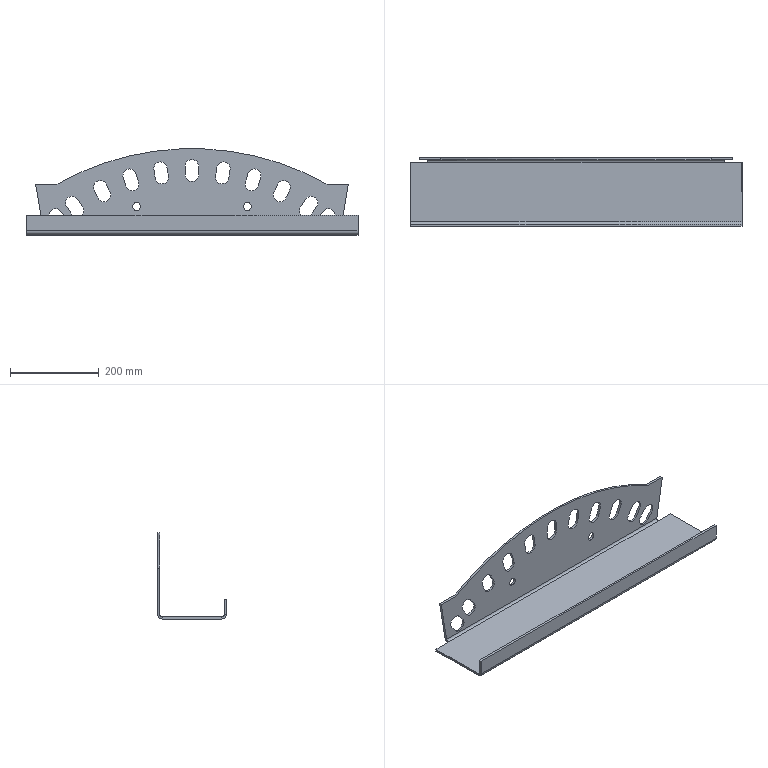Part | SolidWorks | features Cut 1, FlatPattern 1, HoleWzd 1, SM3dBend 1, SMBaseFlange 1, SheetMetal 1, Split 1 | 1 solid | 83 faces | box 750 x 155 x 194.999 mm | volume 1173169 mm3 | cylinder 42 | plane 41 | commonest cylinder face diameters 30 x33 18 x4 10 x2 20 x2 1243 x1